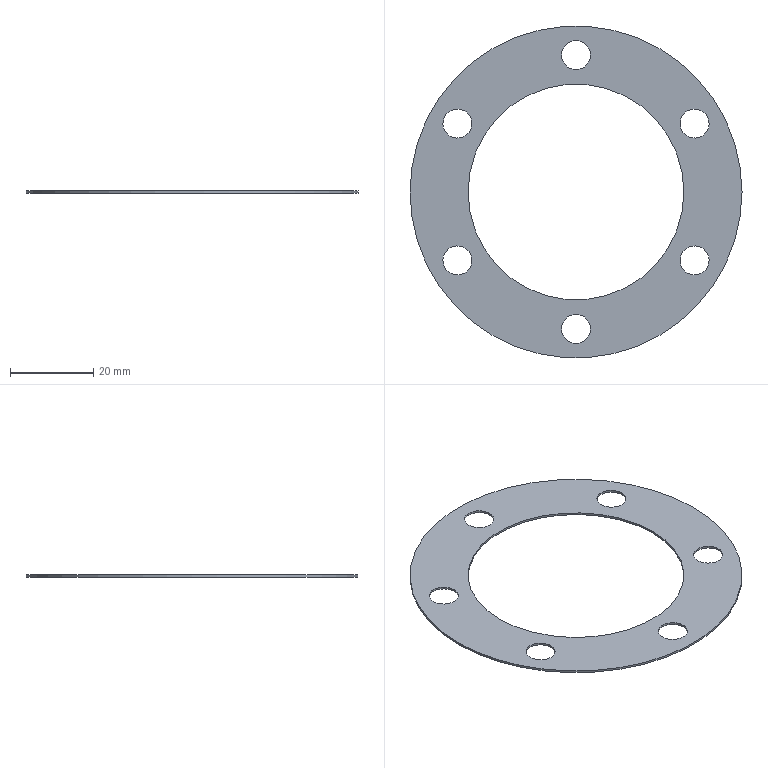Part | NX | features DATUM_CSYS 2, EXTRUDE 1, SKETCH 1 | 1 solid | 10 faces | box 80 x 80 x 0.5 mm | volume 1336 mm3 | cylinder 8 | plane 2 | commonest cylinder face diameters 7 x6 52 x1 80 x1
STEP:
#1=CARTESIAN_POINT('',(-26.829,19.531,0.5));
#2=VERTEX_POINT('',#1);
#3=CARTESIAN_POINT('',(-28.579,16.5,0.5));
#4=DIRECTION('',(0.,0.,1.));
#5=DIRECTION('',(0.5,0.866,0.));
#6=AXIS2_PLACEMENT_3D('',#3,#4,#5);
#7=CIRCLE('',#6,3.5);
#8=EDGE_CURVE('',#2,#2,#7,.T.);
#9=ORIENTED_EDGE('',*,*,#8,.T.);
#10=EDGE_LOOP('',(#9));
#11=FACE_BOUND('',#10,.T.);
#12=CARTESIAN_POINT('',(-26.829,19.531,0.));
#13=VERTEX_POINT('',#12);
#14=CARTESIAN_POINT('',(-28.579,16.5,0.));
#15=DIRECTION('',(0.,0.,1.));
#16=DIRECTION('',(0.5,0.866,0.));
#17=AXIS2_PLACEMENT_3D('',#14,#15,#16);
#18=CIRCLE('',#17,3.5);
#19=EDGE_CURVE('',#13,#13,#18,.T.);
#20=ORIENTED_EDGE('',*,*,#19,.F.);
#21=EDGE_LOOP('',(#20));
#22=FACE_BOUND('',#21,.T.);
#23=CARTESIAN_POINT('',(-28.579,16.5,0.5));
#24=DIRECTION('',(0.,0.,-1.));
#25=DIRECTION('',(-1.,0.,0.));
#26=AXIS2_PLACEMENT_3D('',#23,#24,#25);
#27=CYLINDRICAL_SURFACE('',#26,3.5);
#28=ADVANCED_FACE('',(#11,#22),#27,.F.);
#29=CARTESIAN_POINT('',(26.,0.,0.5));
#30=VERTEX_POINT('',#29);
#31=CARTESIAN_POINT('',(0.,0.,0.5));
#32=DIRECTION('',(0.,0.,1.));
#33=DIRECTION('',(1.,0.,0.));
#34=AXIS2_PLACEMENT_3D('',#31,#32,#33);
#35=CIRCLE('',#34,26.);
#36=EDGE_CURVE('',#30,#30,#35,.T.);
#37=ORIENTED_EDGE('',*,*,#36,.T.);
#38=EDGE_LOOP('',(#37));
#39=FACE_BOUND('',#38,.T.);
#40=CARTESIAN_POINT('',(26.,0.,0.));
#41=VERTEX_POINT('',#40);
#42=CARTESIAN_POINT('',(0.,0.,0.));
#43=DIRECTION('',(0.,0.,1.));
#44=DIRECTION('',(1.,0.,0.));
#45=AXIS2_PLACEMENT_3D('',#42,#43,#44);
#46=CIRCLE('',#45,26.);
#47=EDGE_CURVE('',#41,#41,#46,.T.);
#48=ORIENTED_EDGE('',*,*,#47,.F.);
#49=EDGE_LOOP('',(#48));
#50=FACE_BOUND('',#49,.T.);
#51=CARTESIAN_POINT('',(0.,0.,0.5));
#52=DIRECTION('',(0.,0.,-1.));
#53=DIRECTION('',(-1.,0.,0.));
#54=AXIS2_PLACEMENT_3D('',#51,#52,#53);
#55=CYLINDRICAL_SURFACE('',#54,26.);
#56=ADVANCED_FACE('',(#39,#50),#55,.F.);
#57=CARTESIAN_POINT('',(-3.5,-33.,0.5));
#58=VERTEX_POINT('',#57);
#59=CARTESIAN_POINT('',(0.,-33.,0.5));
#60=DIRECTION('',(0.,0.,1.));
#61=DIRECTION('',(-1.,0.,0.));
#62=AXIS2_PLACEMENT_3D('',#59,#60,#61);
#63=CIRCLE('',#62,3.5);
#64=EDGE_CURVE('',#58,#58,#63,.T.);
#65=ORIENTED_EDGE('',*,*,#64,.T.);
#66=EDGE_LOOP('',(#65));
#67=FACE_BOUND('',#66,.T.);
#68=CARTESIAN_POINT('',(-3.5,-33.,0.));
#69=VERTEX_POINT('',#68);
#70=CARTESIAN_POINT('',(0.,-33.,0.));
#71=DIRECTION('',(0.,0.,1.));
#72=DIRECTION('',(-1.,0.,0.));
#73=AXIS2_PLACEMENT_3D('',#70,#71,#72);
#74=CIRCLE('',#73,3.5);
#75=EDGE_CURVE('',#69,#69,#74,.T.);
#76=ORIENTED_EDGE('',*,*,#75,.F.);
#77=EDGE_LOOP('',(#76));
#78=FACE_BOUND('',#77,.T.);
#79=CARTESIAN_POINT('',(0.,-33.,0.5));
#80=DIRECTION('',(0.,0.,-1.));
#81=DIRECTION('',(-1.,0.,0.));
#82=AXIS2_PLACEMENT_3D('',#79,#80,#81);
#83=CYLINDRICAL_SURFACE('',#82,3.5);
#84=ADVANCED_FACE('',(#67,#78),#83,.F.);
#85=CARTESIAN_POINT('',(3.5,33.,0.5));
#86=VERTEX_POINT('',#85);
#87=CARTESIAN_POINT('',(0.,33.,0.5));
#88=DIRECTION('',(0.,0.,1.));
#89=DIRECTION('',(1.,0.,0.));
#90=AXIS2_PLACEMENT_3D('',#87,#88,#89);
#91=CIRCLE('',#90,3.5);
#92=EDGE_CURVE('',#86,#86,#91,.T.);
#93=ORIENTED_EDGE('',*,*,#92,.T.);
#94=EDGE_LOOP('',(#93));
#95=FACE_BOUND('',#94,.T.);
#96=CARTESIAN_POINT('',(3.5,33.,0.));
#97=VERTEX_POINT('',#96);
#98=CARTESIAN_POINT('',(0.,33.,0.));
#99=DIRECTION('',(0.,0.,1.));
#100=DIRECTION('',(1.,0.,0.));
#101=AXIS2_PLACEMENT_3D('',#98,#99,#100);
#102=CIRCLE('',#101,3.5);
#103=EDGE_CURVE('',#97,#97,#102,.T.);
#104=ORIENTED_EDGE('',*,*,#103,.F.);
#105=EDGE_LOOP('',(#104));
#106=FACE_BOUND('',#105,.T.);
#107=CARTESIAN_POINT('',(0.,33.,0.5));
#108=DIRECTION('',(0.,0.,-1.));
#109=DIRECTION('',(-1.,0.,0.));
#110=AXIS2_PLACEMENT_3D('',#107,#108,#109);
#111=CYLINDRICAL_SURFACE('',#110,3.5);
#112=ADVANCED_FACE('',(#95,#106),#111,.F.);
#113=CARTESIAN_POINT('',(26.829,-19.531,0.5));
#114=VERTEX_POINT('',#113);
#115=CARTESIAN_POINT('',(28.579,-16.5,0.5));
#116=DIRECTION('',(0.,0.,1.));
#117=DIRECTION('',(-0.5,-0.866,0.));
#118=AXIS2_PLACEMENT_3D('',#115,#116,#117);
#119=CIRCLE('',#118,3.5);
#120=EDGE_CURVE('',#114,#114,#119,.T.);
#121=ORIENTED_EDGE('',*,*,#120,.T.);
#122=EDGE_LOOP('',(#121));
#123=FACE_BOUND('',#122,.T.);
#124=CARTESIAN_POINT('',(26.829,-19.531,0.));
#125=VERTEX_POINT('',#124);
#126=CARTESIAN_POINT('',(28.579,-16.5,0.));
#127=DIRECTION('',(0.,0.,1.));
#128=DIRECTION('',(-0.5,-0.866,0.));
#129=AXIS2_PLACEMENT_3D('',#126,#127,#128);
#130=CIRCLE('',#129,3.5);
#131=EDGE_CURVE('',#125,#125,#130,.T.);
#132=ORIENTED_EDGE('',*,*,#131,.F.);
#133=EDGE_LOOP('',(#132));
#134=FACE_BOUND('',#133,.T.);
#135=CARTESIAN_POINT('',(28.579,-16.5,0.5));
#136=DIRECTION('',(0.,0.,-1.));
#137=DIRECTION('',(-1.,0.,0.));
#138=AXIS2_PLACEMENT_3D('',#135,#136,#137);
#139=CYLINDRICAL_SURFACE('',#138,3.5);
#140=ADVANCED_FACE('',(#123,#134),#139,.F.);
#141=CARTESIAN_POINT('',(30.329,13.469,0.5));
#142=VERTEX_POINT('',#141);
#143=CARTESIAN_POINT('',(28.579,16.5,0.5));
#144=DIRECTION('',(0.,0.,1.));
#145=DIRECTION('',(0.5,-0.866,0.));
#146=AXIS2_PLACEMENT_3D('',#143,#144,#145);
#147=CIRCLE('',#146,3.5);
#148=EDGE_CURVE('',#142,#142,#147,.T.);
#149=ORIENTED_EDGE('',*,*,#148,.T.);
#150=EDGE_LOOP('',(#149));
#151=FACE_BOUND('',#150,.T.);
#152=CARTESIAN_POINT('',(30.329,13.469,0.));
#153=VERTEX_POINT('',#152);
#154=CARTESIAN_POINT('',(28.579,16.5,0.));
#155=DIRECTION('',(0.,0.,1.));
#156=DIRECTION('',(0.5,-0.866,0.));
#157=AXIS2_PLACEMENT_3D('',#154,#155,#156);
#158=CIRCLE('',#157,3.5);
#159=EDGE_CURVE('',#153,#153,#158,.T.);
#160=ORIENTED_EDGE('',*,*,#159,.F.);
#161=EDGE_LOOP('',(#160));
#162=FACE_BOUND('',#161,.T.);
#163=CARTESIAN_POINT('',(28.579,16.5,0.5));
#164=DIRECTION('',(0.,0.,-1.));
#165=DIRECTION('',(-1.,0.,0.));
#166=AXIS2_PLACEMENT_3D('',#163,#164,#165);
#167=CYLINDRICAL_SURFACE('',#166,3.5);
#168=ADVANCED_FACE('',(#151,#162),#167,.F.);
#169=CARTESIAN_POINT('',(40.,0.,0.5));
#170=VERTEX_POINT('',#169);
#171=CARTESIAN_POINT('',(0.,0.,0.5));
#172=DIRECTION('',(0.,0.,1.));
#173=DIRECTION('',(1.,0.,0.));
#174=AXIS2_PLACEMENT_3D('',#171,#172,#173);
#175=CIRCLE('',#174,40.);
#176=EDGE_CURVE('',#170,#170,#175,.T.);
#177=ORIENTED_EDGE('',*,*,#176,.F.);
#178=EDGE_LOOP('',(#177));
#179=FACE_BOUND('',#178,.T.);
#180=CARTESIAN_POINT('',(40.,0.,0.));
#181=VERTEX_POINT('',#180);
#182=CARTESIAN_POINT('',(0.,0.,0.));
#183=DIRECTION('',(0.,0.,1.));
#184=DIRECTION('',(1.,0.,0.));
#185=AXIS2_PLACEMENT_3D('',#182,#183,#184);
#186=CIRCLE('',#185,40.);
#187=EDGE_CURVE('',#181,#181,#186,.T.);
#188=ORIENTED_EDGE('',*,*,#187,.T.);
#189=EDGE_LOOP('',(#188));
#190=FACE_BOUND('',#189,.T.);
#191=CARTESIAN_POINT('',(0.,0.,0.5));
#192=DIRECTION('',(0.,0.,-1.));
#193=DIRECTION('',(-1.,0.,0.));
#194=AXIS2_PLACEMENT_3D('',#191,#192,#193);
#195=CYLINDRICAL_SURFACE('',#194,40.);
#196=ADVANCED_FACE('',(#179,#190),#195,.T.);
#197=CARTESIAN_POINT('',(-30.329,-13.469,0.5));
#198=VERTEX_POINT('',#197);
#199=CARTESIAN_POINT('',(-28.579,-16.5,0.5));
#200=DIRECTION('',(0.,0.,1.));
#201=DIRECTION('',(-0.5,0.866,0.));
#202=AXIS2_PLACEMENT_3D('',#199,#200,#201);
#203=CIRCLE('',#202,3.5);
#204=EDGE_CURVE('',#198,#198,#203,.T.);
#205=ORIENTED_EDGE('',*,*,#204,.T.);
#206=EDGE_LOOP('',(#205));
#207=FACE_BOUND('',#206,.T.);
#208=CARTESIAN_POINT('',(-30.329,-13.469,0.));
#209=VERTEX_POINT('',#208);
#210=CARTESIAN_POINT('',(-28.579,-16.5,0.));
#211=DIRECTION('',(0.,0.,1.));
#212=DIRECTION('',(-0.5,0.866,0.));
#213=AXIS2_PLACEMENT_3D('',#210,#211,#212);
#214=CIRCLE('',#213,3.5);
#215=EDGE_CURVE('',#209,#209,#214,.T.);
#216=ORIENTED_EDGE('',*,*,#215,.F.);
#217=EDGE_LOOP('',(#216));
#218=FACE_BOUND('',#217,.T.);
#219=CARTESIAN_POINT('',(-28.579,-16.5,0.5));
#220=DIRECTION('',(0.,0.,-1.));
#221=DIRECTION('',(-1.,0.,0.));
#222=AXIS2_PLACEMENT_3D('',#219,#220,#221);
#223=CYLINDRICAL_SURFACE('',#222,3.5);
#224=ADVANCED_FACE('',(#207,#218),#223,.F.);
#225=ORIENTED_EDGE('',*,*,#176,.T.);
#226=EDGE_LOOP('',(#225));
#227=FACE_BOUND('',#226,.T.);
#228=ORIENTED_EDGE('',*,*,#148,.F.);
#229=EDGE_LOOP('',(#228));
#230=FACE_BOUND('',#229,.T.);
#231=ORIENTED_EDGE('',*,*,#120,.F.);
#232=EDGE_LOOP('',(#231));
#233=FACE_BOUND('',#232,.T.);
#234=ORIENTED_EDGE('',*,*,#92,.F.);
#235=EDGE_LOOP('',(#234));
#236=FACE_BOUND('',#235,.T.);
#237=ORIENTED_EDGE('',*,*,#64,.F.);
#238=EDGE_LOOP('',(#237));
#239=FACE_BOUND('',#238,.T.);
#240=ORIENTED_EDGE('',*,*,#36,.F.);
#241=EDGE_LOOP('',(#240));
#242=FACE_BOUND('',#241,.T.);
#243=ORIENTED_EDGE('',*,*,#8,.F.);
#244=EDGE_LOOP('',(#243));
#245=FACE_BOUND('',#244,.T.);
#246=ORIENTED_EDGE('',*,*,#204,.F.);
#247=EDGE_LOOP('',(#246));
#248=FACE_BOUND('',#247,.T.);
#249=CARTESIAN_POINT('',(14.289,8.25,0.5));
#250=DIRECTION('',(0.,0.,1.));
#251=DIRECTION('',(1.,0.,0.));
#252=AXIS2_PLACEMENT_3D('',#249,#250,#251);
#253=PLANE('',#252);
#254=ADVANCED_FACE('',(#227,#230,#233,#236,#239,#242,#245,#248),#253,.T.);
#255=ORIENTED_EDGE('',*,*,#187,.F.);
#256=EDGE_LOOP('',(#255));
#257=FACE_BOUND('',#256,.T.);
#258=ORIENTED_EDGE('',*,*,#159,.T.);
#259=EDGE_LOOP('',(#258));
#260=FACE_BOUND('',#259,.T.);
#261=ORIENTED_EDGE('',*,*,#131,.T.);
#262=EDGE_LOOP('',(#261));
#263=FACE_BOUND('',#262,.T.);
#264=ORIENTED_EDGE('',*,*,#103,.T.);
#265=EDGE_LOOP('',(#264));
#266=FACE_BOUND('',#265,.T.);
#267=ORIENTED_EDGE('',*,*,#75,.T.);
#268=EDGE_LOOP('',(#267));
#269=FACE_BOUND('',#268,.T.);
#270=ORIENTED_EDGE('',*,*,#47,.T.);
#271=EDGE_LOOP('',(#270));
#272=FACE_BOUND('',#271,.T.);
#273=ORIENTED_EDGE('',*,*,#19,.T.);
#274=EDGE_LOOP('',(#273));
#275=FACE_BOUND('',#274,.T.);
#276=ORIENTED_EDGE('',*,*,#215,.T.);
#277=EDGE_LOOP('',(#276));
#278=FACE_BOUND('',#277,.T.);
#279=CARTESIAN_POINT('',(14.289,8.25,0.));
#280=DIRECTION('',(0.,0.,1.));
#281=DIRECTION('',(1.,0.,0.));
#282=AXIS2_PLACEMENT_3D('',#279,#280,#281);
#283=PLANE('',#282);
#284=ADVANCED_FACE('',(#257,#260,#263,#266,#269,#272,#275,#278),#283,.F.);
#285=CLOSED_SHELL('',(#28,#56,#84,#112,#140,#168,#196,#224,#254,#284));
#286=MANIFOLD_SOLID_BREP('',#285);
#287=(LENGTH_UNIT()NAMED_UNIT(*)SI_UNIT(.MILLI.,.METRE.));
#288=UNCERTAINTY_MEASURE_WITH_UNIT(LENGTH_MEASURE(0.00001),#287,'','');
#289=(NAMED_UNIT(*)PLANE_ANGLE_UNIT()SI_UNIT($,.RADIAN.));
#290=(NAMED_UNIT(*)SI_UNIT($,.STERADIAN.)SOLID_ANGLE_UNIT());
#291=(GEOMETRIC_REPRESENTATION_CONTEXT(3)GLOBAL_UNCERTAINTY_ASSIGNED_CONTEXT((#288))GLOBAL_UNIT_ASSIGNED_CONTEXT((#287,#289,#290))REPRESENTATION_CONTEXT('',''));
#292=ADVANCED_BREP_SHAPE_REPRESENTATION('',(#286),#291);